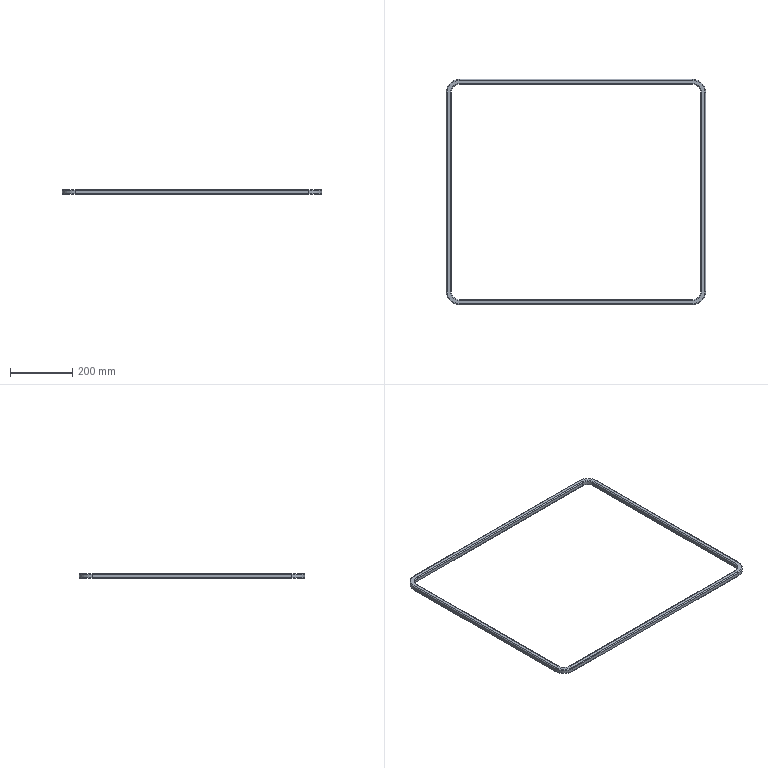Part | STEP file | Front door outer fixing frame lower 01001 | 1 solid | 50 faces | box 836 x 726 x 16 mm | volume 745654 mm3 | cylinder 24 | torus 16 | plane 10 | commonest cylinder face diameters 6 x16 50 x4 82 x4